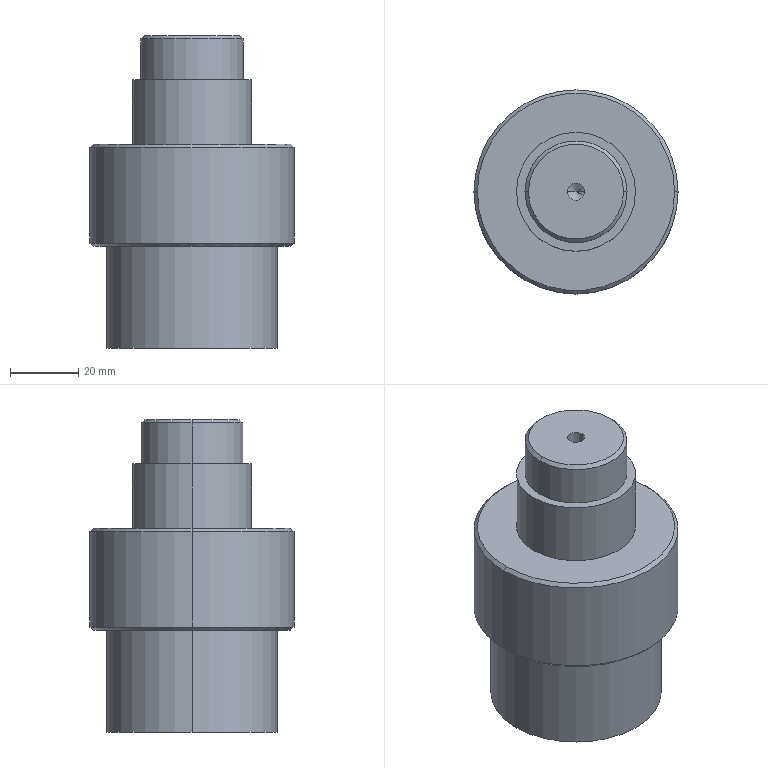Part | SolidWorks | features ICE 6, Chamfer 1, Extrusion 1, HoleWzd 1 | 1 solid | 28 faces | box 60 x 60 x 92 mm | volume 149406 mm3 | cylinder 12 | cone 10 | plane 6 | commonest cylinder face diameters 30 x4 5 x2 35 x2 50 x2 60 x2
STEP:
#1=CARTESIAN_POINT('',(14.,0.,92.));
#2=VERTEX_POINT('',#1);
#3=CARTESIAN_POINT('',(-14.,0.,92.));
#4=VERTEX_POINT('',#3);
#5=CARTESIAN_POINT('',(0.,0.,92.));
#6=DIRECTION('',(0.,0.,1.));
#7=DIRECTION('',(1.,0.,0.));
#8=AXIS2_PLACEMENT_3D('',#5,#6,#7);
#9=CIRCLE('',#8,14.);
#10=EDGE_CURVE('',#2,#4,#9,.T.);
#11=ORIENTED_EDGE('',*,*,#10,.F.);
#12=CARTESIAN_POINT('',(15.,0.,91.));
#13=VERTEX_POINT('',#12);
#14=CARTESIAN_POINT('',(14.,0.,92.));
#15=DIRECTION('',(0.7071,0.,-0.7071));
#16=VECTOR('',#15,1000.);
#17=LINE('',#14,#16);
#18=EDGE_CURVE('',#2,#13,#17,.T.);
#19=ORIENTED_EDGE('',*,*,#18,.T.);
#20=CARTESIAN_POINT('',(-15.,0.,91.));
#21=VERTEX_POINT('',#20);
#22=CARTESIAN_POINT('',(0.,0.,91.));
#23=DIRECTION('',(0.,0.,-1.));
#24=DIRECTION('',(1.,0.,0.));
#25=AXIS2_PLACEMENT_3D('',#22,#23,#24);
#26=CIRCLE('',#25,15.);
#27=EDGE_CURVE('',#21,#13,#26,.T.);
#28=ORIENTED_EDGE('',*,*,#27,.F.);
#29=CARTESIAN_POINT('',(-14.,0.,92.));
#30=DIRECTION('',(-0.7071,0.,-0.7071));
#31=VECTOR('',#30,1000.);
#32=LINE('',#29,#31);
#33=EDGE_CURVE('',#4,#21,#32,.T.);
#34=ORIENTED_EDGE('',*,*,#33,.F.);
#35=EDGE_LOOP('',(#11,#19,#28,#34));
#36=FACE_OUTER_BOUND('',#35,.T.);
#37=CARTESIAN_POINT('',(0.,0.,92.));
#38=DIRECTION('',(0.,0.,-1.));
#39=DIRECTION('',(-1.,0.,0.));
#40=AXIS2_PLACEMENT_3D('',#37,#38,#39);
#41=CONICAL_SURFACE('',#40,14.,0.7854);
#42=ADVANCED_FACE('',(#36),#41,.T.);
#43=CARTESIAN_POINT('',(15.,0.,1.));
#44=VERTEX_POINT('',#43);
#45=CARTESIAN_POINT('',(-15.,0.,1.));
#46=VERTEX_POINT('',#45);
#47=CARTESIAN_POINT('',(0.,0.,1.));
#48=DIRECTION('',(0.,0.,-1.));
#49=DIRECTION('',(1.,0.,0.));
#50=AXIS2_PLACEMENT_3D('',#47,#48,#49);
#51=CIRCLE('',#50,15.);
#52=EDGE_CURVE('',#44,#46,#51,.T.);
#53=ORIENTED_EDGE('',*,*,#52,.F.);
#54=CARTESIAN_POINT('',(16.,0.,0.));
#55=VERTEX_POINT('',#54);
#56=CARTESIAN_POINT('',(15.,0.,1.));
#57=DIRECTION('',(0.7071,0.,-0.7071));
#58=VECTOR('',#57,1000.);
#59=LINE('',#56,#58);
#60=EDGE_CURVE('',#44,#55,#59,.T.);
#61=ORIENTED_EDGE('',*,*,#60,.T.);
#62=CARTESIAN_POINT('',(-16.,0.,0.));
#63=VERTEX_POINT('',#62);
#64=CARTESIAN_POINT('',(0.,0.,0.));
#65=DIRECTION('',(0.,0.,1.));
#66=DIRECTION('',(1.,0.,0.));
#67=AXIS2_PLACEMENT_3D('',#64,#65,#66);
#68=CIRCLE('',#67,16.);
#69=EDGE_CURVE('',#63,#55,#68,.T.);
#70=ORIENTED_EDGE('',*,*,#69,.F.);
#71=CARTESIAN_POINT('',(-15.,0.,1.));
#72=DIRECTION('',(-0.7071,0.,-0.7071));
#73=VECTOR('',#72,1000.);
#74=LINE('',#71,#73);
#75=EDGE_CURVE('',#46,#63,#74,.T.);
#76=ORIENTED_EDGE('',*,*,#75,.F.);
#77=EDGE_LOOP('',(#53,#61,#70,#76));
#78=FACE_OUTER_BOUND('',#77,.T.);
#79=CARTESIAN_POINT('',(0.,0.,1.));
#80=DIRECTION('',(0.,0.,-1.));
#81=DIRECTION('',(-1.,0.,0.));
#82=AXIS2_PLACEMENT_3D('',#79,#80,#81);
#83=CONICAL_SURFACE('',#82,15.,0.7854);
#84=ADVANCED_FACE('',(#78),#83,.F.);
#85=CARTESIAN_POINT('',(29.,0.,60.));
#86=VERTEX_POINT('',#85);
#87=CARTESIAN_POINT('',(-29.,0.,60.));
#88=VERTEX_POINT('',#87);
#89=CARTESIAN_POINT('',(0.,0.,60.));
#90=DIRECTION('',(0.,0.,1.));
#91=DIRECTION('',(1.,0.,0.));
#92=AXIS2_PLACEMENT_3D('',#89,#90,#91);
#93=CIRCLE('',#92,29.);
#94=EDGE_CURVE('',#86,#88,#93,.T.);
#95=ORIENTED_EDGE('',*,*,#94,.F.);
#96=CARTESIAN_POINT('',(30.,0.,59.));
#97=VERTEX_POINT('',#96);
#98=CARTESIAN_POINT('',(29.,0.,60.));
#99=DIRECTION('',(0.7071,0.,-0.7071));
#100=VECTOR('',#99,1000.);
#101=LINE('',#98,#100);
#102=EDGE_CURVE('',#86,#97,#101,.T.);
#103=ORIENTED_EDGE('',*,*,#102,.T.);
#104=CARTESIAN_POINT('',(-30.,0.,59.));
#105=VERTEX_POINT('',#104);
#106=CARTESIAN_POINT('',(0.,0.,59.));
#107=DIRECTION('',(0.,0.,-1.));
#108=DIRECTION('',(1.,0.,0.));
#109=AXIS2_PLACEMENT_3D('',#106,#107,#108);
#110=CIRCLE('',#109,30.);
#111=EDGE_CURVE('',#105,#97,#110,.T.);
#112=ORIENTED_EDGE('',*,*,#111,.F.);
#113=CARTESIAN_POINT('',(-29.,0.,60.));
#114=DIRECTION('',(-0.7071,0.,-0.7071));
#115=VECTOR('',#114,1000.);
#116=LINE('',#113,#115);
#117=EDGE_CURVE('',#88,#105,#116,.T.);
#118=ORIENTED_EDGE('',*,*,#117,.F.);
#119=EDGE_LOOP('',(#95,#103,#112,#118));
#120=FACE_OUTER_BOUND('',#119,.T.);
#121=CARTESIAN_POINT('',(0.,0.,60.));
#122=DIRECTION('',(0.,0.,-1.));
#123=DIRECTION('',(-1.,0.,0.));
#124=AXIS2_PLACEMENT_3D('',#121,#122,#123);
#125=CONICAL_SURFACE('',#124,29.,0.7854);
#126=ADVANCED_FACE('',(#120),#125,.T.);
#127=CARTESIAN_POINT('',(-29.,0.,30.));
#128=VERTEX_POINT('',#127);
#129=CARTESIAN_POINT('',(29.,0.,30.));
#130=VERTEX_POINT('',#129);
#131=CARTESIAN_POINT('',(0.,0.,30.));
#132=DIRECTION('',(0.,0.,-1.));
#133=DIRECTION('',(1.,0.,0.));
#134=AXIS2_PLACEMENT_3D('',#131,#132,#133);
#135=CIRCLE('',#134,29.);
#136=EDGE_CURVE('',#128,#130,#135,.T.);
#137=ORIENTED_EDGE('',*,*,#136,.F.);
#138=CARTESIAN_POINT('',(-30.,0.,31.));
#139=VERTEX_POINT('',#138);
#140=CARTESIAN_POINT('',(-30.,0.,31.));
#141=DIRECTION('',(-0.7071,0.,0.7071));
#142=VECTOR('',#141,1000.);
#143=LINE('',#140,#142);
#144=EDGE_CURVE('',#128,#139,#143,.T.);
#145=ORIENTED_EDGE('',*,*,#144,.T.);
#146=CARTESIAN_POINT('',(30.,0.,31.));
#147=VERTEX_POINT('',#146);
#148=CARTESIAN_POINT('',(0.,0.,31.));
#149=DIRECTION('',(0.,0.,1.));
#150=DIRECTION('',(1.,0.,0.));
#151=AXIS2_PLACEMENT_3D('',#148,#149,#150);
#152=CIRCLE('',#151,30.);
#153=EDGE_CURVE('',#147,#139,#152,.T.);
#154=ORIENTED_EDGE('',*,*,#153,.F.);
#155=CARTESIAN_POINT('',(30.,0.,31.));
#156=DIRECTION('',(0.7071,0.,0.7071));
#157=VECTOR('',#156,1000.);
#158=LINE('',#155,#157);
#159=EDGE_CURVE('',#130,#147,#158,.T.);
#160=ORIENTED_EDGE('',*,*,#159,.F.);
#161=EDGE_LOOP('',(#137,#145,#154,#160));
#162=FACE_OUTER_BOUND('',#161,.T.);
#163=CARTESIAN_POINT('',(0.,0.,31.));
#164=DIRECTION('',(0.,0.,1.));
#165=DIRECTION('',(1.,0.,0.));
#166=AXIS2_PLACEMENT_3D('',#163,#164,#165);
#167=CONICAL_SURFACE('',#166,30.,0.7854);
#168=ADVANCED_FACE('',(#162),#167,.T.);
#169=CARTESIAN_POINT('',(-2.5,0.,77.));
#170=VERTEX_POINT('',#169);
#171=CARTESIAN_POINT('',(2.5,0.,77.));
#172=VERTEX_POINT('',#171);
#173=CARTESIAN_POINT('',(0.,0.,77.));
#174=DIRECTION('',(0.,0.,1.));
#175=DIRECTION('',(1.,0.,0.));
#176=AXIS2_PLACEMENT_3D('',#173,#174,#175);
#177=CIRCLE('',#176,2.5);
#178=EDGE_CURVE('',#170,#172,#177,.T.);
#179=ORIENTED_EDGE('',*,*,#178,.F.);
#180=CARTESIAN_POINT('',(-2.5,0.,92.));
#181=VERTEX_POINT('',#180);
#182=CARTESIAN_POINT('',(-2.5,0.,92.));
#183=DIRECTION('',(0.,0.,1.));
#184=VECTOR('',#183,1000.);
#185=LINE('',#182,#184);
#186=EDGE_CURVE('',#170,#181,#185,.T.);
#187=ORIENTED_EDGE('',*,*,#186,.T.);
#188=CARTESIAN_POINT('',(2.5,0.,92.));
#189=VERTEX_POINT('',#188);
#190=CARTESIAN_POINT('',(0.,0.,92.));
#191=DIRECTION('',(0.,0.,1.));
#192=DIRECTION('',(1.,0.,0.));
#193=AXIS2_PLACEMENT_3D('',#190,#191,#192);
#194=CIRCLE('',#193,2.5);
#195=EDGE_CURVE('',#181,#189,#194,.T.);
#196=ORIENTED_EDGE('',*,*,#195,.T.);
#197=CARTESIAN_POINT('',(2.5,0.,92.));
#198=DIRECTION('',(0.,0.,1.));
#199=VECTOR('',#198,1000.);
#200=LINE('',#197,#199);
#201=EDGE_CURVE('',#172,#189,#200,.T.);
#202=ORIENTED_EDGE('',*,*,#201,.F.);
#203=EDGE_LOOP('',(#179,#187,#196,#202));
#204=FACE_OUTER_BOUND('',#203,.T.);
#205=CARTESIAN_POINT('',(0.,0.,92.));
#206=DIRECTION('',(0.,0.,1.));
#207=DIRECTION('',(1.,0.,0.));
#208=AXIS2_PLACEMENT_3D('',#205,#206,#207);
#209=CYLINDRICAL_SURFACE('',#208,2.5);
#210=ADVANCED_FACE('',(#204),#209,.F.);
#211=CARTESIAN_POINT('',(0.,0.,75.498));
#212=VERTEX_POINT('',#211);
#213=CARTESIAN_POINT('',(2.5,0.,77.));
#214=DIRECTION('',(0.8572,0.,0.515));
#215=VECTOR('',#214,1000.);
#216=LINE('',#213,#215);
#217=EDGE_CURVE('',#212,#172,#216,.T.);
#218=ORIENTED_EDGE('',*,*,#217,.F.);
#219=CARTESIAN_POINT('',(-2.5,0.,77.));
#220=DIRECTION('',(-0.8572,0.,0.515));
#221=VECTOR('',#220,1000.);
#222=LINE('',#219,#221);
#223=EDGE_CURVE('',#212,#170,#222,.T.);
#224=ORIENTED_EDGE('',*,*,#223,.T.);
#225=ORIENTED_EDGE('',*,*,#178,.T.);
#226=EDGE_LOOP('',(#218,#224,#225));
#227=FACE_OUTER_BOUND('',#226,.T.);
#228=CARTESIAN_POINT('',(0.,0.,77.));
#229=DIRECTION('',(0.,0.,1.));
#230=DIRECTION('',(1.,0.,0.));
#231=AXIS2_PLACEMENT_3D('',#228,#229,#230);
#232=CONICAL_SURFACE('',#231,2.5,1.03);
#233=ADVANCED_FACE('',(#227),#232,.F.);
#234=CARTESIAN_POINT('',(15.,0.,79.));
#235=VERTEX_POINT('',#234);
#236=CARTESIAN_POINT('',(-15.,0.,79.));
#237=VERTEX_POINT('',#236);
#238=CARTESIAN_POINT('',(0.,0.,79.));
#239=DIRECTION('',(0.,0.,1.));
#240=DIRECTION('',(1.,0.,0.));
#241=AXIS2_PLACEMENT_3D('',#238,#239,#240);
#242=CIRCLE('',#241,15.);
#243=EDGE_CURVE('',#235,#237,#242,.T.);
#244=ORIENTED_EDGE('',*,*,#243,.T.);
#245=CARTESIAN_POINT('',(-15.,0.,79.));
#246=DIRECTION('',(0.,0.,1.));
#247=VECTOR('',#246,1000.);
#248=LINE('',#245,#247);
#249=EDGE_CURVE('',#237,#21,#248,.T.);
#250=ORIENTED_EDGE('',*,*,#249,.T.);
#251=ORIENTED_EDGE('',*,*,#27,.T.);
#252=CARTESIAN_POINT('',(15.,0.,79.));
#253=DIRECTION('',(0.,0.,1.));
#254=VECTOR('',#253,1000.);
#255=LINE('',#252,#254);
#256=EDGE_CURVE('',#235,#13,#255,.T.);
#257=ORIENTED_EDGE('',*,*,#256,.F.);
#258=EDGE_LOOP('',(#244,#250,#251,#257));
#259=FACE_OUTER_BOUND('',#258,.T.);
#260=CARTESIAN_POINT('',(0.,0.,79.));
#261=DIRECTION('',(0.,0.,1.));
#262=DIRECTION('',(1.,0.,0.));
#263=AXIS2_PLACEMENT_3D('',#260,#261,#262);
#264=CYLINDRICAL_SURFACE('',#263,15.);
#265=ADVANCED_FACE('',(#259),#264,.T.);
#266=ORIENTED_EDGE('',*,*,#111,.T.);
#267=CARTESIAN_POINT('',(30.,0.,60.));
#268=DIRECTION('',(0.,0.,-1.));
#269=VECTOR('',#268,1000.);
#270=LINE('',#267,#269);
#271=EDGE_CURVE('',#97,#147,#270,.T.);
#272=ORIENTED_EDGE('',*,*,#271,.T.);
#273=ORIENTED_EDGE('',*,*,#153,.T.);
#274=CARTESIAN_POINT('',(-30.,0.,60.));
#275=DIRECTION('',(0.,0.,-1.));
#276=VECTOR('',#275,1000.);
#277=LINE('',#274,#276);
#278=EDGE_CURVE('',#105,#139,#277,.T.);
#279=ORIENTED_EDGE('',*,*,#278,.F.);
#280=EDGE_LOOP('',(#266,#272,#273,#279));
#281=FACE_OUTER_BOUND('',#280,.T.);
#282=CARTESIAN_POINT('',(0.,0.,60.));
#283=DIRECTION('',(0.,0.,-1.));
#284=DIRECTION('',(-1.,0.,0.));
#285=AXIS2_PLACEMENT_3D('',#282,#283,#284);
#286=CYLINDRICAL_SURFACE('',#285,30.);
#287=ADVANCED_FACE('',(#281),#286,.T.);
#288=CARTESIAN_POINT('',(25.,0.,30.));
#289=VERTEX_POINT('',#288);
#290=CARTESIAN_POINT('',(-25.,0.,30.));
#291=VERTEX_POINT('',#290);
#292=CARTESIAN_POINT('',(0.,0.,30.));
#293=DIRECTION('',(0.,0.,1.));
#294=DIRECTION('',(1.,0.,0.));
#295=AXIS2_PLACEMENT_3D('',#292,#293,#294);
#296=CIRCLE('',#295,25.);
#297=EDGE_CURVE('',#289,#291,#296,.T.);
#298=ORIENTED_EDGE('',*,*,#297,.F.);
#299=CARTESIAN_POINT('',(25.,0.,0.));
#300=VERTEX_POINT('',#299);
#301=CARTESIAN_POINT('',(25.,0.,30.));
#302=DIRECTION('',(0.,0.,-1.));
#303=VECTOR('',#302,1000.);
#304=LINE('',#301,#303);
#305=EDGE_CURVE('',#289,#300,#304,.T.);
#306=ORIENTED_EDGE('',*,*,#305,.T.);
#307=CARTESIAN_POINT('',(-25.,0.,0.));
#308=VERTEX_POINT('',#307);
#309=CARTESIAN_POINT('',(0.,0.,0.));
#310=DIRECTION('',(0.,0.,1.));
#311=DIRECTION('',(1.,0.,0.));
#312=AXIS2_PLACEMENT_3D('',#309,#310,#311);
#313=CIRCLE('',#312,25.);
#314=EDGE_CURVE('',#300,#308,#313,.T.);
#315=ORIENTED_EDGE('',*,*,#314,.T.);
#316=CARTESIAN_POINT('',(-25.,0.,30.));
#317=DIRECTION('',(0.,0.,-1.));
#318=VECTOR('',#317,1000.);
#319=LINE('',#316,#318);
#320=EDGE_CURVE('',#291,#308,#319,.T.);
#321=ORIENTED_EDGE('',*,*,#320,.F.);
#322=EDGE_LOOP('',(#298,#306,#315,#321));
#323=FACE_OUTER_BOUND('',#322,.T.);
#324=CARTESIAN_POINT('',(0.,0.,30.));
#325=DIRECTION('',(0.,0.,-1.));
#326=DIRECTION('',(-1.,0.,0.));
#327=AXIS2_PLACEMENT_3D('',#324,#325,#326);
#328=CYLINDRICAL_SURFACE('',#327,25.);
#329=ADVANCED_FACE('',(#323),#328,.T.);
#330=CARTESIAN_POINT('',(15.,0.,30.));
#331=VERTEX_POINT('',#330);
#332=CARTESIAN_POINT('',(-15.,0.,30.));
#333=VERTEX_POINT('',#332);
#334=CARTESIAN_POINT('',(0.,0.,30.));
#335=DIRECTION('',(0.,0.,-1.));
#336=DIRECTION('',(1.,0.,0.));
#337=AXIS2_PLACEMENT_3D('',#334,#335,#336);
#338=CIRCLE('',#337,15.);
#339=EDGE_CURVE('',#331,#333,#338,.T.);
#340=ORIENTED_EDGE('',*,*,#339,.F.);
#341=CARTESIAN_POINT('',(15.,0.,60.));
#342=DIRECTION('',(0.,0.,-1.));
#343=VECTOR('',#342,1000.);
#344=LINE('',#341,#343);
#345=EDGE_CURVE('',#331,#44,#344,.T.);
#346=ORIENTED_EDGE('',*,*,#345,.T.);
#347=ORIENTED_EDGE('',*,*,#52,.T.);
#348=CARTESIAN_POINT('',(-15.,0.,60.));
#349=DIRECTION('',(0.,0.,-1.));
#350=VECTOR('',#349,1000.);
#351=LINE('',#348,#350);
#352=EDGE_CURVE('',#333,#46,#351,.T.);
#353=ORIENTED_EDGE('',*,*,#352,.F.);
#354=EDGE_LOOP('',(#340,#346,#347,#353));
#355=FACE_OUTER_BOUND('',#354,.T.);
#356=CARTESIAN_POINT('',(0.,0.,60.));
#357=DIRECTION('',(0.,0.,-1.));
#358=DIRECTION('',(-1.,0.,0.));
#359=AXIS2_PLACEMENT_3D('',#356,#357,#358);
#360=CYLINDRICAL_SURFACE('',#359,15.);
#361=ADVANCED_FACE('',(#355),#360,.F.);
#362=CARTESIAN_POINT('',(17.5,0.,79.));
#363=VERTEX_POINT('',#362);
#364=CARTESIAN_POINT('',(-17.5,0.,79.));
#365=VERTEX_POINT('',#364);
#366=CARTESIAN_POINT('',(0.,0.,79.));
#367=DIRECTION('',(0.,0.,1.));
#368=DIRECTION('',(1.,0.,0.));
#369=AXIS2_PLACEMENT_3D('',#366,#367,#368);
#370=CIRCLE('',#369,17.5);
#371=EDGE_CURVE('',#363,#365,#370,.T.);
#372=ORIENTED_EDGE('',*,*,#371,.F.);
#373=CARTESIAN_POINT('',(17.5,0.,60.));
#374=VERTEX_POINT('',#373);
#375=CARTESIAN_POINT('',(17.5,0.,92.));
#376=DIRECTION('',(0.,0.,-1.));
#377=VECTOR('',#376,1000.);
#378=LINE('',#375,#377);
#379=EDGE_CURVE('',#363,#374,#378,.T.);
#380=ORIENTED_EDGE('',*,*,#379,.T.);
#381=CARTESIAN_POINT('',(-17.5,0.,60.));
#382=VERTEX_POINT('',#381);
#383=CARTESIAN_POINT('',(0.,0.,60.));
#384=DIRECTION('',(0.,0.,1.));
#385=DIRECTION('',(1.,0.,0.));
#386=AXIS2_PLACEMENT_3D('',#383,#384,#385);
#387=CIRCLE('',#386,17.5);
#388=EDGE_CURVE('',#374,#382,#387,.T.);
#389=ORIENTED_EDGE('',*,*,#388,.T.);
#390=CARTESIAN_POINT('',(-17.5,0.,92.));
#391=DIRECTION('',(0.,0.,-1.));
#392=VECTOR('',#391,1000.);
#393=LINE('',#390,#392);
#394=EDGE_CURVE('',#365,#382,#393,.T.);
#395=ORIENTED_EDGE('',*,*,#394,.F.);
#396=EDGE_LOOP('',(#372,#380,#389,#395));
#397=FACE_OUTER_BOUND('',#396,.T.);
#398=CARTESIAN_POINT('',(0.,0.,92.));
#399=DIRECTION('',(0.,0.,-1.));
#400=DIRECTION('',(-1.,0.,0.));
#401=AXIS2_PLACEMENT_3D('',#398,#399,#400);
#402=CYLINDRICAL_SURFACE('',#401,17.5);
#403=ADVANCED_FACE('',(#397),#402,.T.);
#404=ORIENTED_EDGE('',*,*,#379,.F.);
#405=CARTESIAN_POINT('',(0.,0.,79.));
#406=DIRECTION('',(0.,0.,1.));
#407=DIRECTION('',(1.,0.,0.));
#408=AXIS2_PLACEMENT_3D('',#405,#406,#407);
#409=CIRCLE('',#408,17.5);
#410=EDGE_CURVE('',#365,#363,#409,.T.);
#411=ORIENTED_EDGE('',*,*,#410,.F.);
#412=ORIENTED_EDGE('',*,*,#394,.T.);
#413=CARTESIAN_POINT('',(0.,0.,60.));
#414=DIRECTION('',(0.,0.,1.));
#415=DIRECTION('',(1.,0.,0.));
#416=AXIS2_PLACEMENT_3D('',#413,#414,#415);
#417=CIRCLE('',#416,17.5);
#418=EDGE_CURVE('',#382,#374,#417,.T.);
#419=ORIENTED_EDGE('',*,*,#418,.T.);
#420=EDGE_LOOP('',(#404,#411,#412,#419));
#421=FACE_OUTER_BOUND('',#420,.T.);
#422=CARTESIAN_POINT('',(0.,0.,92.));
#423=DIRECTION('',(0.,0.,-1.));
#424=DIRECTION('',(-1.,0.,0.));
#425=AXIS2_PLACEMENT_3D('',#422,#423,#424);
#426=CYLINDRICAL_SURFACE('',#425,17.5);
#427=ADVANCED_FACE('',(#421),#426,.T.);
#428=ORIENTED_EDGE('',*,*,#345,.F.);
#429=CARTESIAN_POINT('',(0.,0.,30.));
#430=DIRECTION('',(0.,0.,-1.));
#431=DIRECTION('',(1.,0.,0.));
#432=AXIS2_PLACEMENT_3D('',#429,#430,#431);
#433=CIRCLE('',#432,15.);
#434=EDGE_CURVE('',#333,#331,#433,.T.);
#435=ORIENTED_EDGE('',*,*,#434,.F.);
#436=ORIENTED_EDGE('',*,*,#352,.T.);
#437=CARTESIAN_POINT('',(0.,0.,1.));
#438=DIRECTION('',(0.,0.,-1.));
#439=DIRECTION('',(1.,0.,0.));
#440=AXIS2_PLACEMENT_3D('',#437,#438,#439);
#441=CIRCLE('',#440,15.);
#442=EDGE_CURVE('',#46,#44,#441,.T.);
#443=ORIENTED_EDGE('',*,*,#442,.T.);
#444=EDGE_LOOP('',(#428,#435,#436,#443));
#445=FACE_OUTER_BOUND('',#444,.T.);
#446=CARTESIAN_POINT('',(0.,0.,60.));
#447=DIRECTION('',(0.,0.,-1.));
#448=DIRECTION('',(-1.,0.,0.));
#449=AXIS2_PLACEMENT_3D('',#446,#447,#448);
#450=CYLINDRICAL_SURFACE('',#449,15.);
#451=ADVANCED_FACE('',(#445),#450,.F.);
#452=ORIENTED_EDGE('',*,*,#305,.F.);
#453=CARTESIAN_POINT('',(0.,0.,30.));
#454=DIRECTION('',(0.,0.,1.));
#455=DIRECTION('',(1.,0.,0.));
#456=AXIS2_PLACEMENT_3D('',#453,#454,#455);
#457=CIRCLE('',#456,25.);
#458=EDGE_CURVE('',#291,#289,#457,.T.);
#459=ORIENTED_EDGE('',*,*,#458,.F.);
#460=ORIENTED_EDGE('',*,*,#320,.T.);
#461=CARTESIAN_POINT('',(0.,0.,0.));
#462=DIRECTION('',(0.,0.,1.));
#463=DIRECTION('',(1.,0.,0.));
#464=AXIS2_PLACEMENT_3D('',#461,#462,#463);
#465=CIRCLE('',#464,25.);
#466=EDGE_CURVE('',#308,#300,#465,.T.);
#467=ORIENTED_EDGE('',*,*,#466,.T.);
#468=EDGE_LOOP('',(#452,#459,#460,#467));
#469=FACE_OUTER_BOUND('',#468,.T.);
#470=CARTESIAN_POINT('',(0.,0.,30.));
#471=DIRECTION('',(0.,0.,-1.));
#472=DIRECTION('',(-1.,0.,0.));
#473=AXIS2_PLACEMENT_3D('',#470,#471,#472);
#474=CYLINDRICAL_SURFACE('',#473,25.);
#475=ADVANCED_FACE('',(#469),#474,.T.);
#476=ORIENTED_EDGE('',*,*,#69,.T.);
#477=CARTESIAN_POINT('',(0.,0.,0.));
#478=DIRECTION('',(0.,0.,1.));
#479=DIRECTION('',(1.,0.,0.));
#480=AXIS2_PLACEMENT_3D('',#477,#478,#479);
#481=CIRCLE('',#480,16.);
#482=EDGE_CURVE('',#55,#63,#481,.T.);
#483=ORIENTED_EDGE('',*,*,#482,.T.);
#484=EDGE_LOOP('',(#476,#483));
#485=FACE_BOUND('',#484,.T.);
#486=ORIENTED_EDGE('',*,*,#466,.F.);
#487=ORIENTED_EDGE('',*,*,#314,.F.);
#488=EDGE_LOOP('',(#486,#487));
#489=FACE_OUTER_BOUND('',#488,.T.);
#490=CARTESIAN_POINT('',(0.,0.,0.));
#491=DIRECTION('',(0.,0.,1.));
#492=DIRECTION('',(1.,0.,0.));
#493=AXIS2_PLACEMENT_3D('',#490,#491,#492);
#494=PLANE('',#493);
#495=ADVANCED_FACE('',(#485,#489),#494,.F.);
#496=ORIENTED_EDGE('',*,*,#271,.F.);
#497=CARTESIAN_POINT('',(0.,0.,59.));
#498=DIRECTION('',(0.,0.,-1.));
#499=DIRECTION('',(1.,0.,0.));
#500=AXIS2_PLACEMENT_3D('',#497,#498,#499);
#501=CIRCLE('',#500,30.);
#502=EDGE_CURVE('',#97,#105,#501,.T.);
#503=ORIENTED_EDGE('',*,*,#502,.T.);
#504=ORIENTED_EDGE('',*,*,#278,.T.);
#505=CARTESIAN_POINT('',(0.,0.,31.));
#506=DIRECTION('',(0.,0.,1.));
#507=DIRECTION('',(1.,0.,0.));
#508=AXIS2_PLACEMENT_3D('',#505,#506,#507);
#509=CIRCLE('',#508,30.);
#510=EDGE_CURVE('',#139,#147,#509,.T.);
#511=ORIENTED_EDGE('',*,*,#510,.T.);
#512=EDGE_LOOP('',(#496,#503,#504,#511));
#513=FACE_OUTER_BOUND('',#512,.T.);
#514=CARTESIAN_POINT('',(0.,0.,60.));
#515=DIRECTION('',(0.,0.,-1.));
#516=DIRECTION('',(-1.,0.,0.));
#517=AXIS2_PLACEMENT_3D('',#514,#515,#516);
#518=CYLINDRICAL_SURFACE('',#517,30.);
#519=ADVANCED_FACE('',(#513),#518,.T.);
#520=CARTESIAN_POINT('',(0.,0.,60.));
#521=DIRECTION('',(0.,0.,1.));
#522=DIRECTION('',(1.,0.,0.));
#523=AXIS2_PLACEMENT_3D('',#520,#521,#522);
#524=CIRCLE('',#523,29.);
#525=EDGE_CURVE('',#88,#86,#524,.T.);
#526=ORIENTED_EDGE('',*,*,#525,.T.);
#527=ORIENTED_EDGE('',*,*,#94,.T.);
#528=EDGE_LOOP('',(#526,#527));
#529=FACE_OUTER_BOUND('',#528,.T.);
#530=ORIENTED_EDGE('',*,*,#418,.F.);
#531=ORIENTED_EDGE('',*,*,#388,.F.);
#532=EDGE_LOOP('',(#530,#531));
#533=FACE_BOUND('',#532,.T.);
#534=CARTESIAN_POINT('',(0.,0.,60.));
#535=DIRECTION('',(0.,0.,1.));
#536=DIRECTION('',(1.,0.,0.));
#537=AXIS2_PLACEMENT_3D('',#534,#535,#536);
#538=PLANE('',#537);
#539=ADVANCED_FACE('',(#529,#533),#538,.T.);
#540=CARTESIAN_POINT('',(0.,0.,30.));
#541=DIRECTION('',(0.,0.,-1.));
#542=DIRECTION('',(1.,0.,0.));
#543=AXIS2_PLACEMENT_3D('',#540,#541,#542);
#544=CIRCLE('',#543,29.);
#545=EDGE_CURVE('',#130,#128,#544,.T.);
#546=ORIENTED_EDGE('',*,*,#545,.T.);
#547=ORIENTED_EDGE('',*,*,#136,.T.);
#548=EDGE_LOOP('',(#546,#547));
#549=FACE_OUTER_BOUND('',#548,.T.);
#550=ORIENTED_EDGE('',*,*,#458,.T.);
#551=ORIENTED_EDGE('',*,*,#297,.T.);
#552=EDGE_LOOP('',(#550,#551));
#553=FACE_BOUND('',#552,.T.);
#554=CARTESIAN_POINT('',(0.,0.,30.));
#555=DIRECTION('',(0.,0.,1.));
#556=DIRECTION('',(1.,0.,0.));
#557=AXIS2_PLACEMENT_3D('',#554,#555,#556);
#558=PLANE('',#557);
#559=ADVANCED_FACE('',(#549,#553),#558,.F.);
#560=ORIENTED_EDGE('',*,*,#434,.T.);
#561=ORIENTED_EDGE('',*,*,#339,.T.);
#562=EDGE_LOOP('',(#560,#561));
#563=FACE_OUTER_BOUND('',#562,.T.);
#564=CARTESIAN_POINT('',(0.,0.,30.));
#565=DIRECTION('',(0.,0.,1.));
#566=DIRECTION('',(1.,0.,0.));
#567=AXIS2_PLACEMENT_3D('',#564,#565,#566);
#568=PLANE('',#567);
#569=ADVANCED_FACE('',(#563),#568,.F.);
#570=ORIENTED_EDGE('',*,*,#243,.F.);
#571=CARTESIAN_POINT('',(0.,0.,79.));
#572=DIRECTION('',(0.,0.,1.));
#573=DIRECTION('',(1.,0.,0.));
#574=AXIS2_PLACEMENT_3D('',#571,#572,#573);
#575=CIRCLE('',#574,15.);
#576=EDGE_CURVE('',#237,#235,#575,.T.);
#577=ORIENTED_EDGE('',*,*,#576,.F.);
#578=EDGE_LOOP('',(#570,#577));
#579=FACE_BOUND('',#578,.T.);
#580=ORIENTED_EDGE('',*,*,#410,.T.);
#581=ORIENTED_EDGE('',*,*,#371,.T.);
#582=EDGE_LOOP('',(#580,#581));
#583=FACE_OUTER_BOUND('',#582,.T.);
#584=CARTESIAN_POINT('',(0.,0.,79.));
#585=DIRECTION('',(0.,0.,1.));
#586=DIRECTION('',(1.,0.,0.));
#587=AXIS2_PLACEMENT_3D('',#584,#585,#586);
#588=PLANE('',#587);
#589=ADVANCED_FACE('',(#579,#583),#588,.T.);
#590=ORIENTED_EDGE('',*,*,#249,.F.);
#591=ORIENTED_EDGE('',*,*,#576,.T.);
#592=ORIENTED_EDGE('',*,*,#256,.T.);
#593=CARTESIAN_POINT('',(0.,0.,91.));
#594=DIRECTION('',(0.,0.,-1.));
#595=DIRECTION('',(1.,0.,0.));
#596=AXIS2_PLACEMENT_3D('',#593,#594,#595);
#597=CIRCLE('',#596,15.);
#598=EDGE_CURVE('',#13,#21,#597,.T.);
#599=ORIENTED_EDGE('',*,*,#598,.T.);
#600=EDGE_LOOP('',(#590,#591,#592,#599));
#601=FACE_OUTER_BOUND('',#600,.T.);
#602=CARTESIAN_POINT('',(0.,0.,79.));
#603=DIRECTION('',(0.,0.,1.));
#604=DIRECTION('',(1.,0.,0.));
#605=AXIS2_PLACEMENT_3D('',#602,#603,#604);
#606=CYLINDRICAL_SURFACE('',#605,15.);
#607=ADVANCED_FACE('',(#601),#606,.T.);
#608=ORIENTED_EDGE('',*,*,#223,.F.);
#609=ORIENTED_EDGE('',*,*,#217,.T.);
#610=CARTESIAN_POINT('',(0.,0.,77.));
#611=DIRECTION('',(0.,0.,1.));
#612=DIRECTION('',(1.,0.,0.));
#613=AXIS2_PLACEMENT_3D('',#610,#611,#612);
#614=CIRCLE('',#613,2.5);
#615=EDGE_CURVE('',#172,#170,#614,.T.);
#616=ORIENTED_EDGE('',*,*,#615,.T.);
#617=EDGE_LOOP('',(#608,#609,#616));
#618=FACE_OUTER_BOUND('',#617,.T.);
#619=CARTESIAN_POINT('',(0.,0.,77.));
#620=DIRECTION('',(0.,0.,1.));
#621=DIRECTION('',(1.,0.,0.));
#622=AXIS2_PLACEMENT_3D('',#619,#620,#621);
#623=CONICAL_SURFACE('',#622,2.5,1.03);
#624=ADVANCED_FACE('',(#618),#623,.F.);
#625=ORIENTED_EDGE('',*,*,#186,.F.);
#626=ORIENTED_EDGE('',*,*,#615,.F.);
#627=ORIENTED_EDGE('',*,*,#201,.T.);
#628=CARTESIAN_POINT('',(0.,0.,92.));
#629=DIRECTION('',(0.,0.,1.));
#630=DIRECTION('',(1.,0.,0.));
#631=AXIS2_PLACEMENT_3D('',#628,#629,#630);
#632=CIRCLE('',#631,2.5);
#633=EDGE_CURVE('',#189,#181,#632,.T.);
#634=ORIENTED_EDGE('',*,*,#633,.T.);
#635=EDGE_LOOP('',(#625,#626,#627,#634));
#636=FACE_OUTER_BOUND('',#635,.T.);
#637=CARTESIAN_POINT('',(0.,0.,92.));
#638=DIRECTION('',(0.,0.,1.));
#639=DIRECTION('',(1.,0.,0.));
#640=AXIS2_PLACEMENT_3D('',#637,#638,#639);
#641=CYLINDRICAL_SURFACE('',#640,2.5);
#642=ADVANCED_FACE('',(#636),#641,.F.);
#643=CARTESIAN_POINT('',(0.,0.,92.));
#644=DIRECTION('',(0.,0.,1.));
#645=DIRECTION('',(1.,0.,0.));
#646=AXIS2_PLACEMENT_3D('',#643,#644,#645);
#647=CIRCLE('',#646,14.);
#648=EDGE_CURVE('',#4,#2,#647,.T.);
#649=ORIENTED_EDGE('',*,*,#648,.T.);
#650=ORIENTED_EDGE('',*,*,#10,.T.);
#651=EDGE_LOOP('',(#649,#650));
#652=FACE_OUTER_BOUND('',#651,.T.);
#653=ORIENTED_EDGE('',*,*,#633,.F.);
#654=ORIENTED_EDGE('',*,*,#195,.F.);
#655=EDGE_LOOP('',(#653,#654));
#656=FACE_BOUND('',#655,.T.);
#657=CARTESIAN_POINT('',(0.,0.,92.));
#658=DIRECTION('',(0.,0.,1.));
#659=DIRECTION('',(1.,0.,0.));
#660=AXIS2_PLACEMENT_3D('',#657,#658,#659);
#661=PLANE('',#660);
#662=ADVANCED_FACE('',(#652,#656),#661,.T.);
#663=ORIENTED_EDGE('',*,*,#144,.F.);
#664=ORIENTED_EDGE('',*,*,#545,.F.);
#665=ORIENTED_EDGE('',*,*,#159,.T.);
#666=ORIENTED_EDGE('',*,*,#510,.F.);
#667=EDGE_LOOP('',(#663,#664,#665,#666));
#668=FACE_OUTER_BOUND('',#667,.T.);
#669=CARTESIAN_POINT('',(0.,0.,31.));
#670=DIRECTION('',(0.,0.,1.));
#671=DIRECTION('',(1.,0.,0.));
#672=AXIS2_PLACEMENT_3D('',#669,#670,#671);
#673=CONICAL_SURFACE('',#672,30.,0.7854);
#674=ADVANCED_FACE('',(#668),#673,.T.);
#675=ORIENTED_EDGE('',*,*,#102,.F.);
#676=ORIENTED_EDGE('',*,*,#525,.F.);
#677=ORIENTED_EDGE('',*,*,#117,.T.);
#678=ORIENTED_EDGE('',*,*,#502,.F.);
#679=EDGE_LOOP('',(#675,#676,#677,#678));
#680=FACE_OUTER_BOUND('',#679,.T.);
#681=CARTESIAN_POINT('',(0.,0.,60.));
#682=DIRECTION('',(0.,0.,-1.));
#683=DIRECTION('',(-1.,0.,0.));
#684=AXIS2_PLACEMENT_3D('',#681,#682,#683);
#685=CONICAL_SURFACE('',#684,29.,0.7854);
#686=ADVANCED_FACE('',(#680),#685,.T.);
#687=ORIENTED_EDGE('',*,*,#60,.F.);
#688=ORIENTED_EDGE('',*,*,#442,.F.);
#689=ORIENTED_EDGE('',*,*,#75,.T.);
#690=ORIENTED_EDGE('',*,*,#482,.F.);
#691=EDGE_LOOP('',(#687,#688,#689,#690));
#692=FACE_OUTER_BOUND('',#691,.T.);
#693=CARTESIAN_POINT('',(0.,0.,1.));
#694=DIRECTION('',(0.,0.,-1.));
#695=DIRECTION('',(-1.,0.,0.));
#696=AXIS2_PLACEMENT_3D('',#693,#694,#695);
#697=CONICAL_SURFACE('',#696,15.,0.7854);
#698=ADVANCED_FACE('',(#692),#697,.F.);
#699=ORIENTED_EDGE('',*,*,#18,.F.);
#700=ORIENTED_EDGE('',*,*,#648,.F.);
#701=ORIENTED_EDGE('',*,*,#33,.T.);
#702=ORIENTED_EDGE('',*,*,#598,.F.);
#703=EDGE_LOOP('',(#699,#700,#701,#702));
#704=FACE_OUTER_BOUND('',#703,.T.);
#705=CARTESIAN_POINT('',(0.,0.,92.));
#706=DIRECTION('',(0.,0.,-1.));
#707=DIRECTION('',(-1.,0.,0.));
#708=AXIS2_PLACEMENT_3D('',#705,#706,#707);
#709=CONICAL_SURFACE('',#708,14.,0.7854);
#710=ADVANCED_FACE('',(#704),#709,.T.);
#711=CLOSED_SHELL('',(#42,#84,#126,#168,#210,#233,#265,#287,#329,#361,#403,#427,#451,#475,#495,#519,#539,#559,#569,#589,#607,#624,#642,#662,#674,#686,#698,#710));
#712=MANIFOLD_SOLID_BREP('',#711);
#713=CARTESIAN_POINT('',(0.,0.,0.));
#714=DIRECTION('',(0.,0.,1.));
#715=DIRECTION('',(1.,0.,0.));
#716=AXIS2_PLACEMENT_3D('',#713,#714,#715);
#717=(LENGTH_UNIT()NAMED_UNIT(*)SI_UNIT(.MILLI.,.METRE.));
#718=UNCERTAINTY_MEASURE_WITH_UNIT(LENGTH_MEASURE(0.00001),#717,'','');
#719=(NAMED_UNIT(*)PLANE_ANGLE_UNIT()SI_UNIT($,.RADIAN.));
#720=(NAMED_UNIT(*)SI_UNIT($,.STERADIAN.)SOLID_ANGLE_UNIT());
#721=(GEOMETRIC_REPRESENTATION_CONTEXT(3)GLOBAL_UNCERTAINTY_ASSIGNED_CONTEXT((#718))GLOBAL_UNIT_ASSIGNED_CONTEXT((#717,#719,#720))REPRESENTATION_CONTEXT('',''));
#722=ADVANCED_BREP_SHAPE_REPRESENTATION('',(#712,#716),#721);